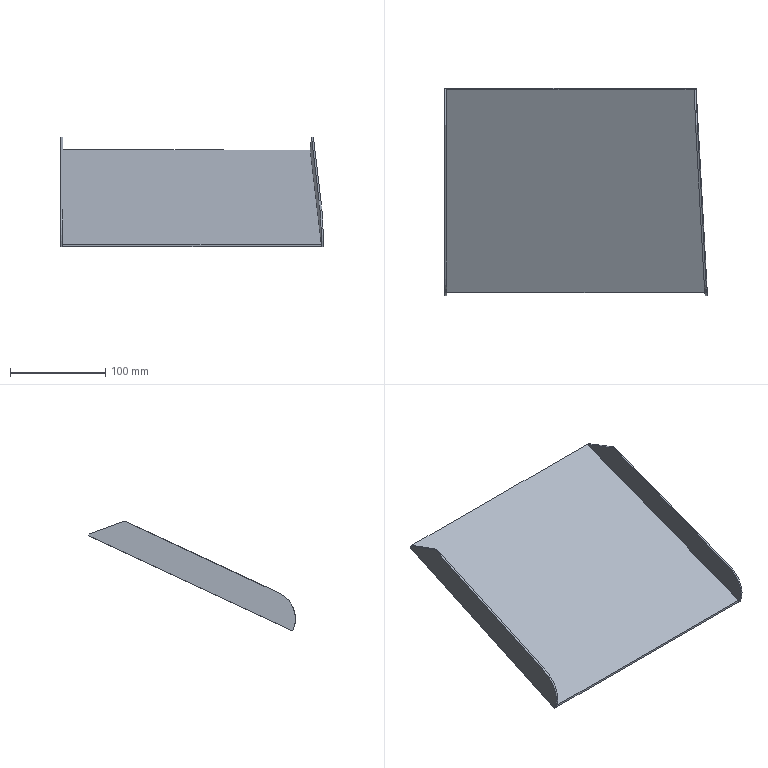Part | NX | features solid 2 | 1 solid | 19 faces | box 276.203 x 217.929 x 115.656 mm | volume 152157 mm3 | plane 14 | spline 3 | cylinder 2 | commonest cylinder face diameters 60 x2
STEP:
#1=CARTESIAN_POINT('',(175.,-625.922,-197.549));
#2=VERTEX_POINT('',#1);
#3=CARTESIAN_POINT('',(42.,-625.841,-197.511));
#4=VERTEX_POINT('',#3);
#5=CARTESIAN_POINT('',(175.,-625.922,-197.549));
#6=CARTESIAN_POINT('',(169.677,-625.901,-197.54));
#7=CARTESIAN_POINT('',(159.282,-625.876,-197.528));
#8=CARTESIAN_POINT('',(140.606,-625.853,-197.517));
#9=CARTESIAN_POINT('',(124.184,-625.841,-197.512));
#10=CARTESIAN_POINT('',(108.509,-625.835,-197.509));
#11=CARTESIAN_POINT('',(94.724,-625.833,-197.508));
#12=CARTESIAN_POINT('',(85.697,-625.833,-197.508));
#13=CARTESIAN_POINT('',(77.967,-625.834,-197.508));
#14=CARTESIAN_POINT('',(70.452,-625.835,-197.509));
#15=CARTESIAN_POINT('',(61.471,-625.836,-197.509));
#16=CARTESIAN_POINT('',(51.352,-625.838,-197.51));
#17=CARTESIAN_POINT('',(45.044,-625.84,-197.511));
#18=CARTESIAN_POINT('',(42.,-625.841,-197.511));
#19=B_SPLINE_CURVE_WITH_KNOTS('',3,(#5,#6,#7,#8,#9,#10,#11,#12,#13,#14,#15,#16,#17,#18),.UNSPECIFIED.,.F.,.F.,(4,1,1,1,1,1,1,1,1,1,1,4),(0.,0.1644,0.2467,0.3289,0.4111,0.4522,0.4933,0.5139,0.5344,0.5755,0.6167,0.6578),.UNSPECIFIED.);
#20=EDGE_CURVE('',#2,#4,#19,.T.);
#21=ORIENTED_EDGE('',*,*,#20,.T.);
#22=CARTESIAN_POINT('',(42.,-840.,-297.376));
#23=VERTEX_POINT('',#22);
#24=CARTESIAN_POINT('',(42.,-651.161,-209.318));
#25=DIRECTION('',(0.,-0.9063,-0.4226));
#26=VECTOR('',#25,1000.);
#27=LINE('',#24,#26);
#28=EDGE_CURVE('',#4,#23,#27,.T.);
#29=ORIENTED_EDGE('',*,*,#28,.T.);
#30=CARTESIAN_POINT('',(314.154,-840.,-297.376));
#31=VERTEX_POINT('',#30);
#32=CARTESIAN_POINT('',(-1209.175,-840.,-297.376));
#33=DIRECTION('',(-1.,0.,0.));
#34=VECTOR('',#33,1000.);
#35=LINE('',#32,#34);
#36=EDGE_CURVE('',#23,#31,#35,.F.);
#37=ORIENTED_EDGE('',*,*,#36,.T.);
#38=CARTESIAN_POINT('',(302.462,-626.273,-197.713));
#39=VERTEX_POINT('',#38);
#40=CARTESIAN_POINT('',(300.114,-583.342,-177.694));
#41=DIRECTION('',(0.04952,-0.9052,-0.4221));
#42=VECTOR('',#41,1000.);
#43=LINE('',#40,#42);
#44=EDGE_CURVE('',#39,#31,#43,.T.);
#45=ORIENTED_EDGE('',*,*,#44,.F.);
#46=CARTESIAN_POINT('',(304.46,-626.183,-197.671));
#47=VERTEX_POINT('',#46);
#48=CARTESIAN_POINT('',(304.46,-626.183,-197.671));
#49=DIRECTION('',(0.9988,0.04488,0.02093));
#50=VECTOR('',#49,1000.);
#51=LINE('',#48,#50);
#52=EDGE_CURVE('',#39,#47,#51,.T.);
#53=ORIENTED_EDGE('',*,*,#52,.T.);
#54=CARTESIAN_POINT('',(216.122,-626.165,-197.663));
#55=VERTEX_POINT('',#54);
#56=CARTESIAN_POINT('',(304.46,-626.183,-197.671));
#57=CARTESIAN_POINT('',(275.014,-626.177,-197.668));
#58=CARTESIAN_POINT('',(245.568,-626.171,-197.666));
#59=CARTESIAN_POINT('',(216.122,-626.165,-197.663));
#60=B_SPLINE_CURVE_WITH_KNOTS('',3,(#56,#57,#58,#59),.UNSPECIFIED.,.F.,.F.,(4,4),(0.,1.),.UNSPECIFIED.);
#61=EDGE_CURVE('',#55,#47,#60,.F.);
#62=ORIENTED_EDGE('',*,*,#61,.F.);
#63=CARTESIAN_POINT('',(195.,-625.944,-197.56));
#64=VERTEX_POINT('',#63);
#65=CARTESIAN_POINT('',(216.122,-626.165,-197.663));
#66=CARTESIAN_POINT('',(215.65,-626.083,-197.624));
#67=CARTESIAN_POINT('',(214.731,-625.959,-197.567));
#68=CARTESIAN_POINT('',(213.668,-625.905,-197.541));
#69=CARTESIAN_POINT('',(212.831,-625.929,-197.553));
#70=CARTESIAN_POINT('',(212.163,-625.951,-197.563));
#71=CARTESIAN_POINT('',(211.498,-625.981,-197.577));
#72=CARTESIAN_POINT('',(211.127,-625.986,-197.579));
#73=CARTESIAN_POINT('',(210.177,-625.985,-197.579));
#74=CARTESIAN_POINT('',(209.524,-625.979,-197.576));
#75=CARTESIAN_POINT('',(208.862,-625.974,-197.573));
#76=CARTESIAN_POINT('',(207.982,-625.964,-197.569));
#77=CARTESIAN_POINT('',(207.108,-625.953,-197.564));
#78=CARTESIAN_POINT('',(206.325,-625.941,-197.558));
#79=CARTESIAN_POINT('',(205.907,-625.934,-197.555));
#80=CARTESIAN_POINT('',(205.509,-625.927,-197.551));
#81=CARTESIAN_POINT('',(205.433,-625.925,-197.551));
#82=CARTESIAN_POINT('',(205.2,-625.922,-197.549));
#83=CARTESIAN_POINT('',(204.805,-625.918,-197.547));
#84=CARTESIAN_POINT('',(204.094,-625.913,-197.545));
#85=CARTESIAN_POINT('',(203.062,-625.91,-197.544));
#86=CARTESIAN_POINT('',(201.427,-625.911,-197.544));
#87=CARTESIAN_POINT('',(198.91,-625.92,-197.548));
#88=CARTESIAN_POINT('',(196.388,-625.935,-197.555));
#89=CARTESIAN_POINT('',(195.,-625.944,-197.56));
#90=B_SPLINE_CURVE_WITH_KNOTS('',3,(#65,#66,#67,#68,#69,#70,#71,#72,#73,#74,#75,#76,#77,#78,#79,#80,#81,#82,#83,#84,#85,#86,#87,#88,#89),.UNSPECIFIED.,.F.,.F.,(4,1,1,1,1,1,1,1,1,1,1,1,1,1,1,1,1,1,1,1,1,1,4),(0.,0.0625,0.125,0.1562,0.1875,0.2188,0.25,0.2812,0.3125,0.3438,0.375,0.4375,0.4688,0.4844,0.5,0.5156,0.5312,0.5625,0.625,0.6875,0.75,0.875,1.),.UNSPECIFIED.);
#91=EDGE_CURVE('',#64,#55,#90,.F.);
#92=ORIENTED_EDGE('',*,*,#91,.F.);
#93=CARTESIAN_POINT('',(195.,-625.844,-197.513));
#94=VERTEX_POINT('',#93);
#95=CARTESIAN_POINT('',(195.,-651.161,-209.318));
#96=DIRECTION('',(0.,0.9063,0.4226));
#97=VECTOR('',#96,1000.);
#98=LINE('',#95,#97);
#99=EDGE_CURVE('',#64,#94,#98,.T.);
#100=ORIENTED_EDGE('',*,*,#99,.T.);
#101=CARTESIAN_POINT('',(175.,-625.82,-197.502));
#102=VERTEX_POINT('',#101);
#103=CARTESIAN_POINT('',(195.,-625.844,-197.513));
#104=CARTESIAN_POINT('',(192.494,-625.861,-197.521));
#105=CARTESIAN_POINT('',(185.827,-625.853,-197.517));
#106=CARTESIAN_POINT('',(175.,-625.82,-197.502));
#107=B_SPLINE_CURVE_WITH_KNOTS('',3,(#103,#104,#105,#106),.UNSPECIFIED.,.F.,.F.,(4,4),(0.,1.),.UNSPECIFIED.);
#108=EDGE_CURVE('',#94,#102,#107,.T.);
#109=ORIENTED_EDGE('',*,*,#108,.T.);
#110=CARTESIAN_POINT('',(175.,-622.634,-196.016));
#111=DIRECTION('',(0.,-0.9063,-0.4226));
#112=VECTOR('',#111,1000.);
#113=LINE('',#110,#112);
#114=EDGE_CURVE('',#102,#2,#113,.T.);
#115=ORIENTED_EDGE('',*,*,#114,.T.);
#116=EDGE_LOOP('',(#21,#29,#37,#45,#53,#62,#92,#100,#109,#115));
#117=FACE_BOUND('',#116,.T.);
#118=CARTESIAN_POINT('',(-1209.175,-651.161,-209.318));
#119=DIRECTION('',(0.,-0.4226,0.9063));
#120=DIRECTION('',(1.,0.,0.));
#121=AXIS2_PLACEMENT_3D('',#118,#119,#120);
#122=PLANE('',#121);
#123=ADVANCED_FACE('',(#117),#122,.T.);
#124=ORIENTED_EDGE('',*,*,#36,.F.);
#125=CARTESIAN_POINT('',(42.,-840.,-299.582));
#126=VERTEX_POINT('',#125);
#127=CARTESIAN_POINT('',(42.,-840.,-720.));
#128=DIRECTION('',(0.,0.,1.));
#129=VECTOR('',#128,1000.);
#130=LINE('',#127,#129);
#131=EDGE_CURVE('',#23,#126,#130,.F.);
#132=ORIENTED_EDGE('',*,*,#131,.T.);
#133=CARTESIAN_POINT('',(314.2,-840.,-299.582));
#134=VERTEX_POINT('',#133);
#135=CARTESIAN_POINT('',(-1209.175,-840.,-299.582));
#136=DIRECTION('',(-1.,0.,0.));
#137=VECTOR('',#136,1000.);
#138=LINE('',#135,#137);
#139=EDGE_CURVE('',#126,#134,#138,.F.);
#140=ORIENTED_EDGE('',*,*,#139,.T.);
#141=CARTESIAN_POINT('',(322.659,-840.,-703.26));
#142=DIRECTION('',(-0.02095,0.,0.9998));
#143=VECTOR('',#142,1000.);
#144=LINE('',#141,#143);
#145=EDGE_CURVE('',#31,#134,#144,.F.);
#146=ORIENTED_EDGE('',*,*,#145,.F.);
#147=EDGE_LOOP('',(#124,#132,#140,#146));
#148=FACE_BOUND('',#147,.T.);
#149=CARTESIAN_POINT('',(-476.248,-840.,-720.));
#150=DIRECTION('',(0.,1.,0.));
#151=DIRECTION('',(-1.,0.,0.));
#152=AXIS2_PLACEMENT_3D('',#149,#150,#151);
#153=PLANE('',#152);
#154=ADVANCED_FACE('',(#148),#153,.F.);
#155=CARTESIAN_POINT('',(40.,-625.842,-197.512));
#156=VERTEX_POINT('',#155);
#157=CARTESIAN_POINT('',(40.,-624.996,-199.324));
#158=VERTEX_POINT('',#157);
#159=CARTESIAN_POINT('',(40.,-625.842,-197.512));
#160=DIRECTION('',(0.,0.4226,-0.9063));
#161=VECTOR('',#160,1000.);
#162=LINE('',#159,#161);
#163=EDGE_CURVE('',#156,#158,#162,.T.);
#164=ORIENTED_EDGE('',*,*,#163,.F.);
#165=CARTESIAN_POINT('',(42.,-625.842,-197.512));
#166=CARTESIAN_POINT('',(41.333,-625.842,-197.512));
#167=CARTESIAN_POINT('',(40.667,-625.842,-197.512));
#168=CARTESIAN_POINT('',(40.,-625.842,-197.512));
#169=B_SPLINE_CURVE_WITH_KNOTS('',3,(#165,#166,#167,#168),.UNSPECIFIED.,.F.,.F.,(4,4),(0.,1.),.UNSPECIFIED.);
#170=EDGE_CURVE('',#156,#4,#169,.F.);
#171=ORIENTED_EDGE('',*,*,#170,.T.);
#172=ORIENTED_EDGE('',*,*,#20,.F.);
#173=CARTESIAN_POINT('',(175.,-625.076,-199.362));
#174=VERTEX_POINT('',#173);
#175=CARTESIAN_POINT('',(175.,-625.076,-199.362));
#176=CARTESIAN_POINT('',(175.,-625.358,-198.758));
#177=CARTESIAN_POINT('',(175.,-625.64,-198.153));
#178=CARTESIAN_POINT('',(175.,-625.922,-197.549));
#179=B_SPLINE_CURVE_WITH_KNOTS('',3,(#175,#176,#177,#178),.UNSPECIFIED.,.F.,.F.,(4,4),(0.,1.),.UNSPECIFIED.);
#180=EDGE_CURVE('',#2,#174,#179,.F.);
#181=ORIENTED_EDGE('',*,*,#180,.T.);
#182=CARTESIAN_POINT('',(175.,-625.076,-199.362));
#183=CARTESIAN_POINT('',(169.603,-625.056,-199.352));
#184=CARTESIAN_POINT('',(159.032,-625.03,-199.34));
#185=CARTESIAN_POINT('',(139.985,-625.007,-199.329));
#186=CARTESIAN_POINT('',(123.219,-624.995,-199.324));
#187=CARTESIAN_POINT('',(107.199,-624.99,-199.321));
#188=CARTESIAN_POINT('',(93.112,-624.988,-199.321));
#189=CARTESIAN_POINT('',(83.866,-624.988,-199.321));
#190=CARTESIAN_POINT('',(75.985,-624.989,-199.321));
#191=CARTESIAN_POINT('',(68.474,-624.99,-199.321));
#192=CARTESIAN_POINT('',(59.458,-624.991,-199.322));
#193=CARTESIAN_POINT('',(49.337,-624.993,-199.323));
#194=CARTESIAN_POINT('',(43.037,-624.995,-199.324));
#195=CARTESIAN_POINT('',(40.,-624.996,-199.324));
#196=B_SPLINE_CURVE_WITH_KNOTS('',3,(#182,#183,#184,#185,#186,#187,#188,#189,#190,#191,#192,#193,#194,#195),.UNSPECIFIED.,.F.,.F.,(4,1,1,1,1,1,1,1,1,1,1,4),(0.,0.1667,0.2501,0.3334,0.4168,0.4585,0.5001,0.521,0.5418,0.5835,0.6252,0.6668),.UNSPECIFIED.);
#197=EDGE_CURVE('',#174,#158,#196,.T.);
#198=ORIENTED_EDGE('',*,*,#197,.T.);
#199=EDGE_LOOP('',(#164,#171,#172,#181,#198));
#200=FACE_BOUND('',#199,.T.);
#201=CARTESIAN_POINT('',(175.,-625.922,-197.549));
#202=CARTESIAN_POINT('',(175.,-625.076,-199.362));
#203=CARTESIAN_POINT('',(169.603,-625.901,-197.54));
#204=CARTESIAN_POINT('',(169.603,-625.056,-199.352));
#205=CARTESIAN_POINT('',(159.032,-625.876,-197.528));
#206=CARTESIAN_POINT('',(159.032,-625.03,-199.34));
#207=CARTESIAN_POINT('',(139.985,-625.852,-197.517));
#208=CARTESIAN_POINT('',(139.985,-625.007,-199.329));
#209=CARTESIAN_POINT('',(123.219,-625.84,-197.511));
#210=CARTESIAN_POINT('',(123.219,-624.995,-199.324));
#211=CARTESIAN_POINT('',(107.199,-625.835,-197.509));
#212=CARTESIAN_POINT('',(107.199,-624.99,-199.321));
#213=CARTESIAN_POINT('',(93.112,-625.833,-197.508));
#214=CARTESIAN_POINT('',(93.112,-624.988,-199.321));
#215=CARTESIAN_POINT('',(83.866,-625.833,-197.508));
#216=CARTESIAN_POINT('',(83.866,-624.988,-199.321));
#217=CARTESIAN_POINT('',(75.985,-625.834,-197.508));
#218=CARTESIAN_POINT('',(75.985,-624.989,-199.321));
#219=CARTESIAN_POINT('',(68.474,-625.835,-197.509));
#220=CARTESIAN_POINT('',(68.474,-624.99,-199.321));
#221=CARTESIAN_POINT('',(59.458,-625.836,-197.509));
#222=CARTESIAN_POINT('',(59.458,-624.991,-199.322));
#223=CARTESIAN_POINT('',(49.337,-625.839,-197.51));
#224=CARTESIAN_POINT('',(49.337,-624.993,-199.323));
#225=CARTESIAN_POINT('',(43.037,-625.84,-197.511));
#226=CARTESIAN_POINT('',(43.037,-624.995,-199.324));
#227=CARTESIAN_POINT('',(40.,-625.842,-197.512));
#228=CARTESIAN_POINT('',(40.,-624.996,-199.324));
#229=B_SPLINE_SURFACE_WITH_KNOTS('',3,1,((#201,#202),(#203,#204),(#205,#206),(#207,#208),(#209,#210),(#211,#212),(#213,#214),(#215,#216),(#217,#218),(#219,#220),(#221,#222),(#223,#224),(#225,#226),(#227,#228)),.SURF_OF_LINEAR_EXTRUSION.,.F.,.F.,.F.,(4,1,1,1,1,1,1,1,1,1,1,4),(2,2),(0.,0.1667,0.2501,0.3334,0.4168,0.4585,0.5001,0.521,0.5418,0.5835,0.6252,0.6668),(0.,1.),.UNSPECIFIED.);
#230=ADVANCED_FACE('',(#200),#229,.F.);
#231=CARTESIAN_POINT('',(40.,-840.,-299.582));
#232=VERTEX_POINT('',#231);
#233=CARTESIAN_POINT('',(40.,-650.315,-211.131));
#234=DIRECTION('',(0.,-0.9063,-0.4226));
#235=VECTOR('',#234,1000.);
#236=LINE('',#233,#235);
#237=EDGE_CURVE('',#158,#232,#236,.T.);
#238=ORIENTED_EDGE('',*,*,#237,.F.);
#239=ORIENTED_EDGE('',*,*,#197,.F.);
#240=CARTESIAN_POINT('',(175.,-624.975,-199.314));
#241=VERTEX_POINT('',#240);
#242=CARTESIAN_POINT('',(175.,-621.788,-197.829));
#243=DIRECTION('',(0.,-0.9063,-0.4226));
#244=VECTOR('',#243,1000.);
#245=LINE('',#242,#244);
#246=EDGE_CURVE('',#241,#174,#245,.T.);
#247=ORIENTED_EDGE('',*,*,#246,.F.);
#248=CARTESIAN_POINT('',(195.,-624.999,-199.326));
#249=VERTEX_POINT('',#248);
#250=CARTESIAN_POINT('',(195.,-624.999,-199.326));
#251=CARTESIAN_POINT('',(192.494,-625.016,-199.334));
#252=CARTESIAN_POINT('',(185.827,-625.008,-199.33));
#253=CARTESIAN_POINT('',(175.,-624.975,-199.314));
#254=B_SPLINE_CURVE_WITH_KNOTS('',3,(#250,#251,#252,#253),.UNSPECIFIED.,.F.,.F.,(4,4),(0.,1.),.UNSPECIFIED.);
#255=EDGE_CURVE('',#249,#241,#254,.T.);
#256=ORIENTED_EDGE('',*,*,#255,.F.);
#257=CARTESIAN_POINT('',(195.,-625.099,-199.372));
#258=VERTEX_POINT('',#257);
#259=CARTESIAN_POINT('',(195.,-650.315,-211.131));
#260=DIRECTION('',(0.,0.9063,0.4226));
#261=VECTOR('',#260,1000.);
#262=LINE('',#259,#261);
#263=EDGE_CURVE('',#258,#249,#262,.T.);
#264=ORIENTED_EDGE('',*,*,#263,.F.);
#265=CARTESIAN_POINT('',(216.122,-625.32,-199.475));
#266=VERTEX_POINT('',#265);
#267=CARTESIAN_POINT('',(216.122,-625.32,-199.475));
#268=CARTESIAN_POINT('',(215.65,-625.237,-199.437));
#269=CARTESIAN_POINT('',(214.731,-625.114,-199.379));
#270=CARTESIAN_POINT('',(213.668,-625.059,-199.354));
#271=CARTESIAN_POINT('',(212.831,-625.084,-199.365));
#272=CARTESIAN_POINT('',(212.163,-625.106,-199.375));
#273=CARTESIAN_POINT('',(211.498,-625.135,-199.389));
#274=CARTESIAN_POINT('',(211.127,-625.141,-199.392));
#275=CARTESIAN_POINT('',(210.177,-625.14,-199.391));
#276=CARTESIAN_POINT('',(209.524,-625.134,-199.389));
#277=CARTESIAN_POINT('',(208.862,-625.128,-199.386));
#278=CARTESIAN_POINT('',(207.982,-625.119,-199.382));
#279=CARTESIAN_POINT('',(207.108,-625.108,-199.376));
#280=CARTESIAN_POINT('',(206.325,-625.095,-199.371));
#281=CARTESIAN_POINT('',(205.907,-625.088,-199.367));
#282=CARTESIAN_POINT('',(205.509,-625.081,-199.364));
#283=CARTESIAN_POINT('',(205.433,-625.08,-199.364));
#284=CARTESIAN_POINT('',(205.2,-625.077,-199.362));
#285=CARTESIAN_POINT('',(204.805,-625.072,-199.36));
#286=CARTESIAN_POINT('',(204.094,-625.068,-199.358));
#287=CARTESIAN_POINT('',(203.062,-625.065,-199.357));
#288=CARTESIAN_POINT('',(201.427,-625.066,-199.357));
#289=CARTESIAN_POINT('',(198.91,-625.074,-199.361));
#290=CARTESIAN_POINT('',(196.388,-625.089,-199.368));
#291=CARTESIAN_POINT('',(195.,-625.099,-199.372));
#292=B_SPLINE_CURVE_WITH_KNOTS('',3,(#267,#268,#269,#270,#271,#272,#273,#274,#275,#276,#277,#278,#279,#280,#281,#282,#283,#284,#285,#286,#287,#288,#289,#290,#291),.UNSPECIFIED.,.F.,.F.,(4,1,1,1,1,1,1,1,1,1,1,1,1,1,1,1,1,1,1,1,1,1,4),(0.,0.0625,0.125,0.1562,0.1875,0.2188,0.25,0.2812,0.3125,0.3438,0.375,0.4375,0.4688,0.4844,0.5,0.5156,0.5312,0.5625,0.625,0.6875,0.75,0.875,1.),.UNSPECIFIED.);
#293=EDGE_CURVE('',#258,#266,#292,.F.);
#294=ORIENTED_EDGE('',*,*,#293,.T.);
#295=CARTESIAN_POINT('',(304.207,-625.338,-199.484));
#296=VERTEX_POINT('',#295);
#297=CARTESIAN_POINT('',(304.207,-625.338,-199.484));
#298=CARTESIAN_POINT('',(274.845,-625.332,-199.481));
#299=CARTESIAN_POINT('',(245.484,-625.326,-199.478));
#300=CARTESIAN_POINT('',(216.122,-625.32,-199.475));
#301=B_SPLINE_CURVE_WITH_KNOTS('',3,(#297,#298,#299,#300),.UNSPECIFIED.,.F.,.F.,(4,4),(0.002864,1.),.UNSPECIFIED.);
#302=EDGE_CURVE('',#266,#296,#301,.F.);
#303=ORIENTED_EDGE('',*,*,#302,.T.);
#304=CARTESIAN_POINT('',(304.46,-625.338,-199.484));
#305=VERTEX_POINT('',#304);
#306=CARTESIAN_POINT('',(304.46,-625.338,-199.484));
#307=DIRECTION('',(-1.,0.0001974,0.00009204));
#308=VECTOR('',#307,1000.);
#309=LINE('',#306,#308);
#310=EDGE_CURVE('',#296,#305,#309,.F.);
#311=ORIENTED_EDGE('',*,*,#310,.T.);
#312=CARTESIAN_POINT('',(316.203,-840.,-299.582));
#313=VERTEX_POINT('',#312);
#314=CARTESIAN_POINT('',(302.111,-582.407,-179.465));
#315=DIRECTION('',(0.04952,-0.9052,-0.4221));
#316=VECTOR('',#315,1000.);
#317=LINE('',#314,#316);
#318=EDGE_CURVE('',#305,#313,#317,.T.);
#319=ORIENTED_EDGE('',*,*,#318,.T.);
#320=CARTESIAN_POINT('',(314.205,-840.09,-299.624));
#321=VERTEX_POINT('',#320);
#322=CARTESIAN_POINT('',(316.203,-840.,-299.582));
#323=DIRECTION('',(0.9988,0.04488,0.02093));
#324=VECTOR('',#323,1000.);
#325=LINE('',#322,#324);
#326=EDGE_CURVE('',#313,#321,#325,.F.);
#327=ORIENTED_EDGE('',*,*,#326,.T.);
#328=CARTESIAN_POINT('',(302.462,-625.427,-199.525));
#329=DIRECTION('',(0.04952,-0.9052,-0.4221));
#330=VECTOR('',#329,1000.);
#331=LINE('',#328,#330);
#332=EDGE_CURVE('',#134,#321,#331,.T.);
#333=ORIENTED_EDGE('',*,*,#332,.F.);
#334=ORIENTED_EDGE('',*,*,#139,.F.);
#335=CARTESIAN_POINT('',(-1209.175,-840.,-299.582));
#336=DIRECTION('',(-1.,0.,0.));
#337=VECTOR('',#336,1000.);
#338=LINE('',#335,#337);
#339=EDGE_CURVE('',#232,#126,#338,.F.);
#340=ORIENTED_EDGE('',*,*,#339,.F.);
#341=EDGE_LOOP('',(#238,#239,#247,#256,#264,#294,#303,#311,#319,#327,#333,#334,#340));
#342=FACE_BOUND('',#341,.T.);
#343=CARTESIAN_POINT('',(-1209.175,-650.315,-211.131));
#344=DIRECTION('',(0.,-0.4226,0.9063));
#345=DIRECTION('',(1.,0.,0.));
#346=AXIS2_PLACEMENT_3D('',#343,#344,#345);
#347=PLANE('',#346);
#348=ADVANCED_FACE('',(#342),#347,.F.);
#349=ORIENTED_EDGE('',*,*,#255,.T.);
#350=CARTESIAN_POINT('',(175.,-625.82,-197.502));
#351=CARTESIAN_POINT('',(175.,-625.538,-198.106));
#352=CARTESIAN_POINT('',(175.,-625.257,-198.71));
#353=CARTESIAN_POINT('',(175.,-624.975,-199.314));
#354=B_SPLINE_CURVE_WITH_KNOTS('',3,(#350,#351,#352,#353),.UNSPECIFIED.,.F.,.F.,(4,4),(0.,1.),.UNSPECIFIED.);
#355=EDGE_CURVE('',#102,#241,#354,.T.);
#356=ORIENTED_EDGE('',*,*,#355,.F.);
#357=ORIENTED_EDGE('',*,*,#108,.F.);
#358=CARTESIAN_POINT('',(195.,-624.999,-199.326));
#359=CARTESIAN_POINT('',(195.,-625.281,-198.721));
#360=CARTESIAN_POINT('',(195.,-625.562,-198.117));
#361=CARTESIAN_POINT('',(195.,-625.844,-197.513));
#362=B_SPLINE_CURVE_WITH_KNOTS('',3,(#358,#359,#360,#361),.UNSPECIFIED.,.F.,.F.,(4,4),(0.,1.),.UNSPECIFIED.);
#363=EDGE_CURVE('',#94,#249,#362,.F.);
#364=ORIENTED_EDGE('',*,*,#363,.T.);
#365=EDGE_LOOP('',(#349,#356,#357,#364));
#366=FACE_BOUND('',#365,.T.);
#367=CARTESIAN_POINT('',(195.,-625.844,-197.513));
#368=CARTESIAN_POINT('',(195.,-624.999,-199.326));
#369=CARTESIAN_POINT('',(192.494,-625.861,-197.521));
#370=CARTESIAN_POINT('',(192.494,-625.016,-199.334));
#371=CARTESIAN_POINT('',(185.827,-625.853,-197.517));
#372=CARTESIAN_POINT('',(185.827,-625.008,-199.33));
#373=CARTESIAN_POINT('',(175.,-625.82,-197.502));
#374=CARTESIAN_POINT('',(175.,-624.975,-199.314));
#375=B_SPLINE_SURFACE_WITH_KNOTS('',3,1,((#367,#368),(#369,#370),(#371,#372),(#373,#374)),.SURF_OF_LINEAR_EXTRUSION.,.F.,.F.,.F.,(4,4),(2,2),(0.,1.),(0.,1.),.PIECEWISE_BEZIER_KNOTS.);
#376=ADVANCED_FACE('',(#366),#375,.F.);
#377=ORIENTED_EDGE('',*,*,#246,.T.);
#378=ORIENTED_EDGE('',*,*,#180,.F.);
#379=ORIENTED_EDGE('',*,*,#114,.F.);
#380=ORIENTED_EDGE('',*,*,#355,.T.);
#381=EDGE_LOOP('',(#377,#378,#379,#380));
#382=FACE_BOUND('',#381,.T.);
#383=CARTESIAN_POINT('',(175.,-622.634,-196.016));
#384=DIRECTION('',(1.,0.,0.));
#385=DIRECTION('',(0.,1.,0.));
#386=AXIS2_PLACEMENT_3D('',#383,#384,#385);
#387=PLANE('',#386);
#388=ADVANCED_FACE('',(#382),#387,.F.);
#389=ORIENTED_EDGE('',*,*,#237,.T.);
#390=CARTESIAN_POINT('',(40.,-825.489,-259.715));
#391=VERTEX_POINT('',#390);
#392=CARTESIAN_POINT('',(40.,-812.811,-286.904));
#393=DIRECTION('',(-1.,0.,0.));
#394=DIRECTION('',(0.,-1.,0.));
#395=AXIS2_PLACEMENT_3D('',#392,#393,#394);
#396=CIRCLE('',#395,30.);
#397=EDGE_CURVE('',#232,#391,#396,.T.);
#398=ORIENTED_EDGE('',*,*,#397,.T.);
#399=CARTESIAN_POINT('',(40.,-663.051,-183.969));
#400=VERTEX_POINT('',#399);
#401=CARTESIAN_POINT('',(40.,-637.675,-172.135));
#402=DIRECTION('',(0.,-0.9063,-0.4226));
#403=VECTOR('',#402,1000.);
#404=LINE('',#401,#403);
#405=EDGE_CURVE('',#400,#391,#404,.T.);
#406=ORIENTED_EDGE('',*,*,#405,.F.);
#407=CARTESIAN_POINT('',(40.,-624.513,-197.996));
#408=DIRECTION('',(0.,-0.9397,0.342));
#409=VECTOR('',#408,1000.);
#410=LINE('',#407,#409);
#411=EDGE_CURVE('',#400,#156,#410,.F.);
#412=ORIENTED_EDGE('',*,*,#411,.T.);
#413=ORIENTED_EDGE('',*,*,#163,.T.);
#414=EDGE_LOOP('',(#389,#398,#406,#412,#413));
#415=FACE_BOUND('',#414,.T.);
#416=CARTESIAN_POINT('',(40.,-651.161,-209.318));
#417=DIRECTION('',(1.,0.,0.));
#418=DIRECTION('',(0.,1.,0.));
#419=AXIS2_PLACEMENT_3D('',#416,#417,#418);
#420=PLANE('',#419);
#421=ADVANCED_FACE('',(#415),#420,.F.);
#422=ORIENTED_EDGE('',*,*,#318,.F.);
#423=CARTESIAN_POINT('',(304.46,-626.183,-197.671));
#424=DIRECTION('',(0.,-0.4226,0.9063));
#425=VECTOR('',#424,1000.);
#426=LINE('',#423,#425);
#427=EDGE_CURVE('',#47,#305,#426,.F.);
#428=ORIENTED_EDGE('',*,*,#427,.F.);
#429=CARTESIAN_POINT('',(305.846,-663.362,-184.113));
#430=VERTEX_POINT('',#429);
#431=CARTESIAN_POINT('',(305.846,-663.362,-184.113));
#432=DIRECTION('',(-0.03502,0.9389,-0.3424));
#433=VECTOR('',#432,1000.);
#434=LINE('',#431,#433);
#435=EDGE_CURVE('',#47,#430,#434,.F.);
#436=ORIENTED_EDGE('',*,*,#435,.T.);
#437=CARTESIAN_POINT('',(314.717,-825.523,-259.73));
#438=VERTEX_POINT('',#437);
#439=CARTESIAN_POINT('',(304.46,-638.016,-172.294));
#440=DIRECTION('',(0.04952,-0.9052,-0.4221));
#441=VECTOR('',#440,1000.);
#442=LINE('',#439,#441);
#443=EDGE_CURVE('',#430,#438,#442,.T.);
#444=ORIENTED_EDGE('',*,*,#443,.T.);
#445=CARTESIAN_POINT('',(314.717,-812.844,-286.919));
#446=DIRECTION('',(-0.9988,-0.04488,-0.02093));
#447=DIRECTION('',(0.04489,-0.999,0.));
#448=AXIS2_PLACEMENT_3D('',#445,#446,#447);
#449=CIRCLE('',#448,30.);
#450=EDGE_CURVE('',#438,#313,#449,.F.);
#451=ORIENTED_EDGE('',*,*,#450,.T.);
#452=EDGE_LOOP('',(#422,#428,#436,#444,#451));
#453=FACE_BOUND('',#452,.T.);
#454=CARTESIAN_POINT('',(302.111,-583.252,-177.652));
#455=DIRECTION('',(0.9988,0.04488,0.02093));
#456=DIRECTION('',(-0.04489,0.999,0.));
#457=AXIS2_PLACEMENT_3D('',#454,#455,#456);
#458=PLANE('',#457);
#459=ADVANCED_FACE('',(#453),#458,.T.);
#460=ORIENTED_EDGE('',*,*,#302,.F.);
#461=CARTESIAN_POINT('',(216.122,-625.32,-199.475));
#462=CARTESIAN_POINT('',(216.122,-625.602,-198.871));
#463=CARTESIAN_POINT('',(216.122,-625.884,-198.267));
#464=CARTESIAN_POINT('',(216.122,-626.165,-197.663));
#465=B_SPLINE_CURVE_WITH_KNOTS('',3,(#461,#462,#463,#464),.UNSPECIFIED.,.F.,.F.,(4,4),(0.,1.),.UNSPECIFIED.);
#466=EDGE_CURVE('',#55,#266,#465,.F.);
#467=ORIENTED_EDGE('',*,*,#466,.F.);
#468=ORIENTED_EDGE('',*,*,#61,.T.);
#469=ORIENTED_EDGE('',*,*,#427,.T.);
#470=ORIENTED_EDGE('',*,*,#310,.F.);
#471=EDGE_LOOP('',(#460,#467,#468,#469,#470));
#472=FACE_BOUND('',#471,.T.);
#473=CARTESIAN_POINT('',(304.46,-626.183,-197.671));
#474=DIRECTION('',(0.0002178,0.9063,0.4226));
#475=DIRECTION('',(0.,-0.4226,0.9063));
#476=AXIS2_PLACEMENT_3D('',#473,#474,#475);
#477=PLANE('',#476);
#478=ADVANCED_FACE('',(#472),#477,.T.);
#479=ORIENTED_EDGE('',*,*,#293,.F.);
#480=CARTESIAN_POINT('',(195.,-625.944,-197.56));
#481=CARTESIAN_POINT('',(195.,-625.662,-198.164));
#482=CARTESIAN_POINT('',(195.,-625.381,-198.768));
#483=CARTESIAN_POINT('',(195.,-625.099,-199.372));
#484=B_SPLINE_CURVE_WITH_KNOTS('',3,(#480,#481,#482,#483),.UNSPECIFIED.,.F.,.F.,(4,4),(0.,1.),.UNSPECIFIED.);
#485=EDGE_CURVE('',#64,#258,#484,.T.);
#486=ORIENTED_EDGE('',*,*,#485,.F.);
#487=ORIENTED_EDGE('',*,*,#91,.T.);
#488=ORIENTED_EDGE('',*,*,#466,.T.);
#489=EDGE_LOOP('',(#479,#486,#487,#488));
#490=FACE_BOUND('',#489,.T.);
#491=CARTESIAN_POINT('',(216.122,-626.165,-197.663));
#492=CARTESIAN_POINT('',(216.122,-625.32,-199.475));
#493=CARTESIAN_POINT('',(215.65,-626.083,-197.624));
#494=CARTESIAN_POINT('',(215.65,-625.237,-199.437));
#495=CARTESIAN_POINT('',(214.731,-625.959,-197.567));
#496=CARTESIAN_POINT('',(214.731,-625.114,-199.379));
#497=CARTESIAN_POINT('',(213.668,-625.905,-197.541));
#498=CARTESIAN_POINT('',(213.668,-625.059,-199.354));
#499=CARTESIAN_POINT('',(212.831,-625.929,-197.553));
#500=CARTESIAN_POINT('',(212.831,-625.084,-199.365));
#501=CARTESIAN_POINT('',(212.163,-625.951,-197.563));
#502=CARTESIAN_POINT('',(212.163,-625.106,-199.375));
#503=CARTESIAN_POINT('',(211.498,-625.981,-197.577));
#504=CARTESIAN_POINT('',(211.498,-625.135,-199.389));
#505=CARTESIAN_POINT('',(211.127,-625.986,-197.579));
#506=CARTESIAN_POINT('',(211.127,-625.141,-199.392));
#507=CARTESIAN_POINT('',(210.177,-625.985,-197.579));
#508=CARTESIAN_POINT('',(210.177,-625.14,-199.391));
#509=CARTESIAN_POINT('',(209.524,-625.979,-197.576));
#510=CARTESIAN_POINT('',(209.524,-625.134,-199.389));
#511=CARTESIAN_POINT('',(208.862,-625.974,-197.573));
#512=CARTESIAN_POINT('',(208.862,-625.128,-199.386));
#513=CARTESIAN_POINT('',(207.982,-625.964,-197.569));
#514=CARTESIAN_POINT('',(207.982,-625.119,-199.382));
#515=CARTESIAN_POINT('',(207.108,-625.953,-197.564));
#516=CARTESIAN_POINT('',(207.108,-625.108,-199.376));
#517=CARTESIAN_POINT('',(206.325,-625.941,-197.558));
#518=CARTESIAN_POINT('',(206.325,-625.095,-199.371));
#519=CARTESIAN_POINT('',(205.907,-625.934,-197.555));
#520=CARTESIAN_POINT('',(205.907,-625.088,-199.367));
#521=CARTESIAN_POINT('',(205.509,-625.927,-197.551));
#522=CARTESIAN_POINT('',(205.509,-625.081,-199.364));
#523=CARTESIAN_POINT('',(205.433,-625.925,-197.551));
#524=CARTESIAN_POINT('',(205.433,-625.08,-199.364));
#525=CARTESIAN_POINT('',(205.2,-625.922,-197.549));
#526=CARTESIAN_POINT('',(205.2,-625.077,-199.362));
#527=CARTESIAN_POINT('',(204.805,-625.918,-197.547));
#528=CARTESIAN_POINT('',(204.805,-625.072,-199.36));
#529=CARTESIAN_POINT('',(204.094,-625.913,-197.545));
#530=CARTESIAN_POINT('',(204.094,-625.068,-199.358));
#531=CARTESIAN_POINT('',(203.062,-625.91,-197.544));
#532=CARTESIAN_POINT('',(203.062,-625.065,-199.357));
#533=CARTESIAN_POINT('',(201.427,-625.911,-197.544));
#534=CARTESIAN_POINT('',(201.427,-625.066,-199.357));
#535=CARTESIAN_POINT('',(198.91,-625.92,-197.548));
#536=CARTESIAN_POINT('',(198.91,-625.074,-199.361));
#537=CARTESIAN_POINT('',(196.388,-625.935,-197.555));
#538=CARTESIAN_POINT('',(196.388,-625.089,-199.368));
#539=CARTESIAN_POINT('',(195.,-625.944,-197.56));
#540=CARTESIAN_POINT('',(195.,-625.099,-199.372));
#541=B_SPLINE_SURFACE_WITH_KNOTS('',3,1,((#491,#492),(#493,#494),(#495,#496),(#497,#498),(#499,#500),(#501,#502),(#503,#504),(#505,#506),(#507,#508),(#509,#510),(#511,#512),(#513,#514),(#515,#516),(#517,#518),(#519,#520),(#521,#522),(#523,#524),(#525,#526),(#527,#528),(#529,#530),(#531,#532),(#533,#534),(#535,#536),(#537,#538),(#539,#540)),.SURF_OF_LINEAR_EXTRUSION.,.F.,.F.,.F.,(4,1,1,1,1,1,1,1,1,1,1,1,1,1,1,1,1,1,1,1,1,1,4),(2,2),(0.,0.0625,0.125,0.1562,0.1875,0.2188,0.25,0.2812,0.3125,0.3438,0.375,0.4375,0.4688,0.4844,0.5,0.5156,0.5312,0.5625,0.625,0.6875,0.75,0.875,1.),(0.,1.),.UNSPECIFIED.);
#542=ADVANCED_FACE('',(#490),#541,.F.);
#543=ORIENTED_EDGE('',*,*,#263,.T.);
#544=ORIENTED_EDGE('',*,*,#363,.F.);
#545=ORIENTED_EDGE('',*,*,#99,.F.);
#546=ORIENTED_EDGE('',*,*,#485,.T.);
#547=EDGE_LOOP('',(#543,#544,#545,#546));
#548=FACE_BOUND('',#547,.T.);
#549=CARTESIAN_POINT('',(195.,-651.161,-209.318));
#550=DIRECTION('',(-1.,0.,0.));
#551=DIRECTION('',(0.,-1.,0.));
#552=AXIS2_PLACEMENT_3D('',#549,#550,#551);
#553=PLANE('',#552);
#554=ADVANCED_FACE('',(#548),#553,.F.);
#555=CARTESIAN_POINT('',(303.849,-663.451,-184.155));
#556=VERTEX_POINT('',#555);
#557=CARTESIAN_POINT('',(312.72,-825.612,-259.772));
#558=VERTEX_POINT('',#557);
#559=CARTESIAN_POINT('',(302.462,-638.106,-172.336));
#560=DIRECTION('',(0.04952,-0.9052,-0.4221));
#561=VECTOR('',#560,1000.);
#562=LINE('',#559,#561);
#563=EDGE_CURVE('',#556,#558,#562,.T.);
#564=ORIENTED_EDGE('',*,*,#563,.T.);
#565=CARTESIAN_POINT('',(314.717,-825.523,-259.73));
#566=DIRECTION('',(0.9988,0.04488,0.02093));
#567=VECTOR('',#566,1000.);
#568=LINE('',#565,#567);
#569=EDGE_CURVE('',#558,#438,#568,.T.);
#570=ORIENTED_EDGE('',*,*,#569,.T.);
#571=ORIENTED_EDGE('',*,*,#443,.F.);
#572=CARTESIAN_POINT('',(305.846,-663.362,-184.113));
#573=DIRECTION('',(-0.9988,-0.04488,-0.02093));
#574=VECTOR('',#573,1000.);
#575=LINE('',#572,#574);
#576=EDGE_CURVE('',#430,#556,#575,.T.);
#577=ORIENTED_EDGE('',*,*,#576,.T.);
#578=EDGE_LOOP('',(#564,#570,#571,#577));
#579=FACE_BOUND('',#578,.T.);
#580=CARTESIAN_POINT('',(304.46,-638.016,-172.294));
#581=DIRECTION('',(0.,0.4226,-0.9063));
#582=DIRECTION('',(0.04952,-0.9052,-0.4221));
#583=AXIS2_PLACEMENT_3D('',#580,#581,#582);
#584=PLANE('',#583);
#585=ADVANCED_FACE('',(#579),#584,.F.);
#586=CARTESIAN_POINT('',(302.413,-624.945,-198.197));
#587=DIRECTION('',(0.03502,-0.9389,0.3424));
#588=VECTOR('',#587,1000.);
#589=LINE('',#586,#588);
#590=EDGE_CURVE('',#556,#39,#589,.F.);
#591=ORIENTED_EDGE('',*,*,#590,.T.);
#592=ORIENTED_EDGE('',*,*,#44,.T.);
#593=ORIENTED_EDGE('',*,*,#145,.T.);
#594=ORIENTED_EDGE('',*,*,#332,.T.);
#595=CARTESIAN_POINT('',(312.72,-812.934,-286.961));
#596=DIRECTION('',(-0.9988,-0.04488,-0.02093));
#597=DIRECTION('',(0.04489,-0.999,0.));
#598=AXIS2_PLACEMENT_3D('',#595,#596,#597);
#599=CIRCLE('',#598,30.);
#600=EDGE_CURVE('',#321,#558,#599,.T.);
#601=ORIENTED_EDGE('',*,*,#600,.T.);
#602=ORIENTED_EDGE('',*,*,#563,.F.);
#603=EDGE_LOOP('',(#591,#592,#593,#594,#601,#602));
#604=FACE_BOUND('',#603,.T.);
#605=CARTESIAN_POINT('',(302.462,-625.427,-199.525));
#606=DIRECTION('',(-0.9988,-0.04488,-0.02093));
#607=DIRECTION('',(0.04489,-0.999,0.));
#608=AXIS2_PLACEMENT_3D('',#605,#606,#607);
#609=PLANE('',#608);
#610=ADVANCED_FACE('',(#604),#609,.T.);
#611=ORIENTED_EDGE('',*,*,#435,.F.);
#612=ORIENTED_EDGE('',*,*,#52,.F.);
#613=ORIENTED_EDGE('',*,*,#590,.F.);
#614=ORIENTED_EDGE('',*,*,#576,.F.);
#615=EDGE_LOOP('',(#611,#612,#613,#614));
#616=FACE_BOUND('',#615,.T.);
#617=CARTESIAN_POINT('',(305.846,-663.362,-184.113));
#618=DIRECTION('',(0.03502,-0.3412,-0.9393));
#619=DIRECTION('',(0.,0.9399,-0.3414));
#620=AXIS2_PLACEMENT_3D('',#617,#618,#619);
#621=PLANE('',#620);
#622=ADVANCED_FACE('',(#616),#621,.F.);
#623=ORIENTED_EDGE('',*,*,#450,.F.);
#624=ORIENTED_EDGE('',*,*,#569,.F.);
#625=ORIENTED_EDGE('',*,*,#600,.F.);
#626=ORIENTED_EDGE('',*,*,#326,.F.);
#627=EDGE_LOOP('',(#623,#624,#625,#626));
#628=FACE_BOUND('',#627,.T.);
#629=CARTESIAN_POINT('',(314.717,-812.844,-286.919));
#630=DIRECTION('',(0.9988,0.04488,0.02093));
#631=DIRECTION('',(-0.04489,0.999,0.));
#632=AXIS2_PLACEMENT_3D('',#629,#630,#631);
#633=CYLINDRICAL_SURFACE('',#632,30.);
#634=ADVANCED_FACE('',(#628),#633,.T.);
#635=ORIENTED_EDGE('',*,*,#405,.T.);
#636=CARTESIAN_POINT('',(42.,-825.489,-259.715));
#637=VERTEX_POINT('',#636);
#638=CARTESIAN_POINT('',(40.,-825.489,-259.715));
#639=DIRECTION('',(1.,0.,0.));
#640=VECTOR('',#639,1000.);
#641=LINE('',#638,#640);
#642=EDGE_CURVE('',#391,#637,#641,.T.);
#643=ORIENTED_EDGE('',*,*,#642,.T.);
#644=CARTESIAN_POINT('',(42.,-663.051,-183.969));
#645=VERTEX_POINT('',#644);
#646=CARTESIAN_POINT('',(42.,-637.675,-172.135));
#647=DIRECTION('',(0.,-0.9063,-0.4226));
#648=VECTOR('',#647,1000.);
#649=LINE('',#646,#648);
#650=EDGE_CURVE('',#645,#637,#649,.T.);
#651=ORIENTED_EDGE('',*,*,#650,.F.);
#652=CARTESIAN_POINT('',(40.,-663.051,-183.969));
#653=DIRECTION('',(1.,0.,0.));
#654=VECTOR('',#653,1000.);
#655=LINE('',#652,#654);
#656=EDGE_CURVE('',#645,#400,#655,.F.);
#657=ORIENTED_EDGE('',*,*,#656,.T.);
#658=EDGE_LOOP('',(#635,#643,#651,#657));
#659=FACE_BOUND('',#658,.T.);
#660=CARTESIAN_POINT('',(40.,-637.675,-172.135));
#661=DIRECTION('',(0.,0.4226,-0.9063));
#662=DIRECTION('',(0.,-0.9063,-0.4226));
#663=AXIS2_PLACEMENT_3D('',#660,#661,#662);
#664=PLANE('',#663);
#665=ADVANCED_FACE('',(#659),#664,.F.);
#666=ORIENTED_EDGE('',*,*,#28,.F.);
#667=CARTESIAN_POINT('',(42.,-625.842,-197.512));
#668=DIRECTION('',(0.,0.9397,-0.342));
#669=VECTOR('',#668,1000.);
#670=LINE('',#667,#669);
#671=EDGE_CURVE('',#4,#645,#670,.F.);
#672=ORIENTED_EDGE('',*,*,#671,.T.);
#673=ORIENTED_EDGE('',*,*,#650,.T.);
#674=CARTESIAN_POINT('',(42.,-812.811,-286.904));
#675=DIRECTION('',(-1.,0.,0.));
#676=DIRECTION('',(0.,-1.,0.));
#677=AXIS2_PLACEMENT_3D('',#674,#675,#676);
#678=CIRCLE('',#677,30.);
#679=EDGE_CURVE('',#637,#126,#678,.F.);
#680=ORIENTED_EDGE('',*,*,#679,.T.);
#681=ORIENTED_EDGE('',*,*,#131,.F.);
#682=EDGE_LOOP('',(#666,#672,#673,#680,#681));
#683=FACE_BOUND('',#682,.T.);
#684=CARTESIAN_POINT('',(42.,-624.996,-199.324));
#685=DIRECTION('',(-1.,0.,0.));
#686=DIRECTION('',(0.,-1.,0.));
#687=AXIS2_PLACEMENT_3D('',#684,#685,#686);
#688=PLANE('',#687);
#689=ADVANCED_FACE('',(#683),#688,.F.);
#690=ORIENTED_EDGE('',*,*,#411,.F.);
#691=ORIENTED_EDGE('',*,*,#656,.F.);
#692=ORIENTED_EDGE('',*,*,#671,.F.);
#693=ORIENTED_EDGE('',*,*,#170,.F.);
#694=EDGE_LOOP('',(#690,#691,#692,#693));
#695=FACE_BOUND('',#694,.T.);
#696=CARTESIAN_POINT('',(40.,-625.842,-197.512));
#697=DIRECTION('',(0.,-0.342,-0.9397));
#698=DIRECTION('',(0.,0.9397,-0.342));
#699=AXIS2_PLACEMENT_3D('',#696,#697,#698);
#700=PLANE('',#699);
#701=ADVANCED_FACE('',(#695),#700,.F.);
#702=ORIENTED_EDGE('',*,*,#397,.F.);
#703=ORIENTED_EDGE('',*,*,#339,.T.);
#704=ORIENTED_EDGE('',*,*,#679,.F.);
#705=ORIENTED_EDGE('',*,*,#642,.F.);
#706=EDGE_LOOP('',(#702,#703,#704,#705));
#707=FACE_BOUND('',#706,.T.);
#708=CARTESIAN_POINT('',(40.,-812.811,-286.904));
#709=DIRECTION('',(-1.,0.,0.));
#710=DIRECTION('',(0.,-1.,0.));
#711=AXIS2_PLACEMENT_3D('',#708,#709,#710);
#712=CYLINDRICAL_SURFACE('',#711,30.);
#713=ADVANCED_FACE('',(#707),#712,.T.);
#714=CLOSED_SHELL('',(#123,#154,#230,#348,#376,#388,#421,#459,#478,#542,#554,#585,#610,#622,#634,#665,#689,#701,#713));
#715=MANIFOLD_SOLID_BREP('',#714);
#716=(LENGTH_UNIT()NAMED_UNIT(*)SI_UNIT(.MILLI.,.METRE.));
#717=UNCERTAINTY_MEASURE_WITH_UNIT(LENGTH_MEASURE(0.05143),#716,'','');
#718=(NAMED_UNIT(*)PLANE_ANGLE_UNIT()SI_UNIT($,.RADIAN.));
#719=(NAMED_UNIT(*)SI_UNIT($,.STERADIAN.)SOLID_ANGLE_UNIT());
#720=(GEOMETRIC_REPRESENTATION_CONTEXT(3)GLOBAL_UNCERTAINTY_ASSIGNED_CONTEXT((#717))GLOBAL_UNIT_ASSIGNED_CONTEXT((#716,#718,#719))REPRESENTATION_CONTEXT('',''));
#721=ADVANCED_BREP_SHAPE_REPRESENTATION('',(#715),#720);